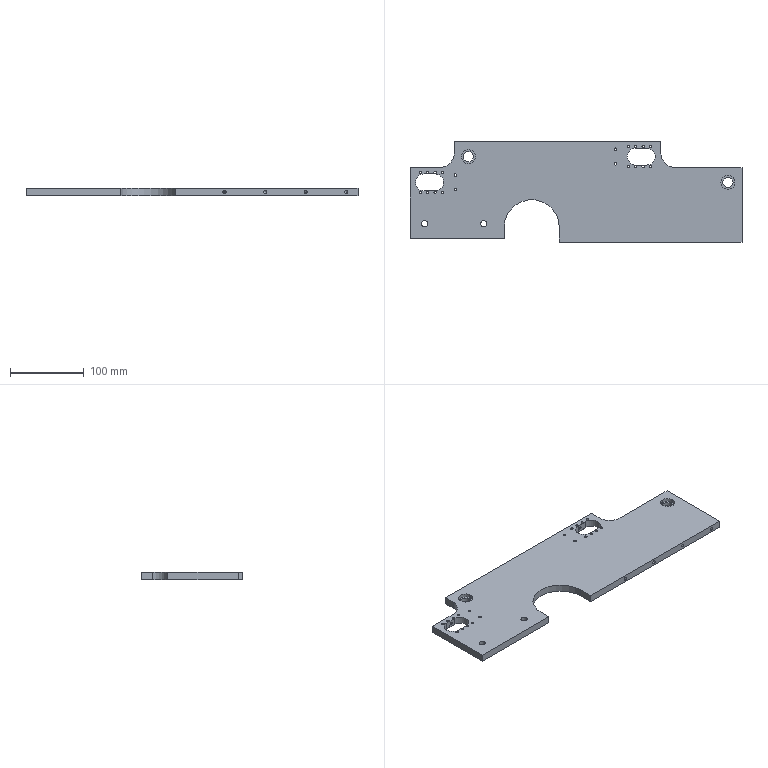Part | STEP file | 08-02 conveyor right baffle | 1 solid | 104 faces | box 450 x 136 x 10 mm | volume 487378 mm3 | cylinder 75 | plane 19 | cone 10 | commonest cylinder face diameters 3.3 x46 4.2 x8 23 x6 8.5 x4 14 x4 19 x4